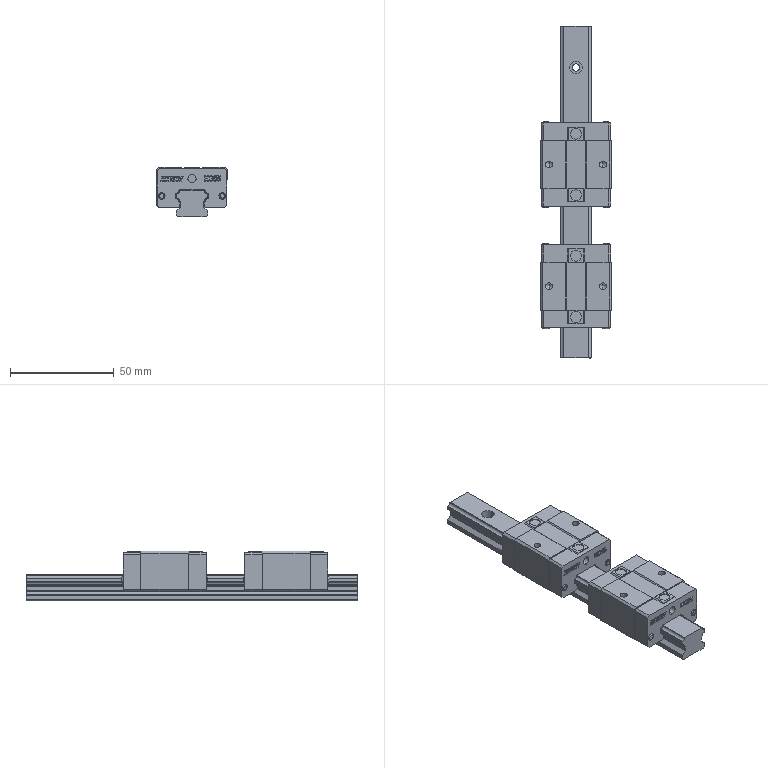Part | SolidWorks | 3 solids | 839 faces | box 34 x 160 x 24 mm | volume 68410 mm3 | plane 545 | cylinder 150 | spline 120 | torus 16 | cone 8 | commonest cylinder face diameters 1.6 x32 2.1 x24 0.6 x19 0.46 x16 3 x13 0.74 x8